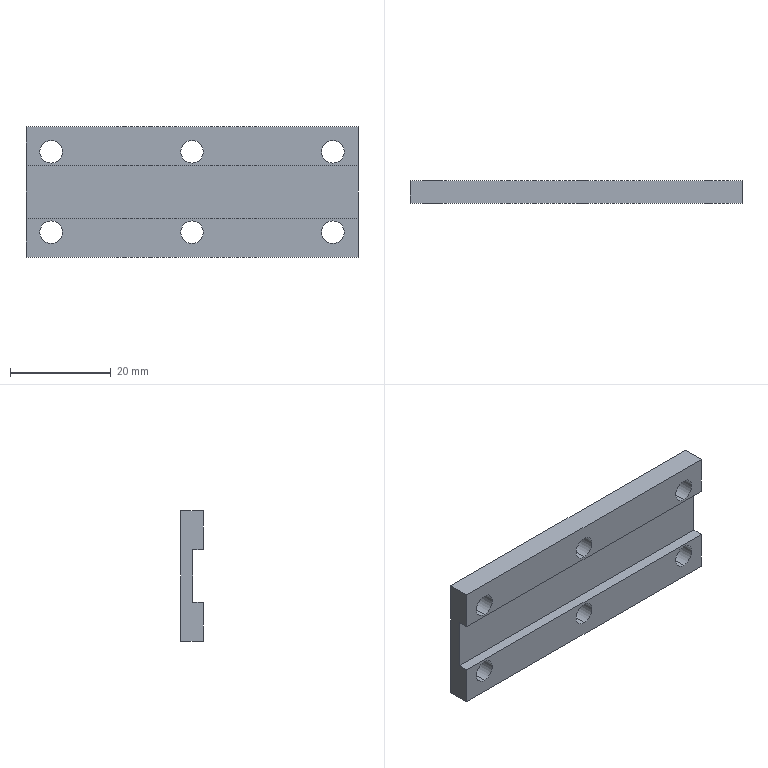Part | SolidWorks | features BaseBody 1 | 1 solid | 22 faces | box 66 x 4.5 x 26 mm | volume 5837 mm3 | cylinder 12 | plane 10 | commonest cylinder face diameters 4.5 x12
STEP:
#1=CARTESIAN_POINT('',(0.,4.7,5.75));
#2=VERTEX_POINT('',#1);
#3=CARTESIAN_POINT('',(0.,4.7,10.25));
#4=VERTEX_POINT('',#3);
#5=CARTESIAN_POINT('',(0.,4.7,8.));
#6=DIRECTION('',(0.,1.,0.));
#7=DIRECTION('',(0.,0.,1.));
#8=AXIS2_PLACEMENT_3D('',#5,#6,#7);
#9=CIRCLE('',#8,2.25);
#10=EDGE_CURVE('',#2,#4,#9,.T.);
#11=ORIENTED_EDGE('',*,*,#10,.F.);
#12=CARTESIAN_POINT('',(0.,9.2,5.75));
#13=VERTEX_POINT('',#12);
#14=CARTESIAN_POINT('',(0.,4.7,5.75));
#15=DIRECTION('',(0.,1.,0.));
#16=VECTOR('',#15,1000.);
#17=LINE('',#14,#16);
#18=EDGE_CURVE('',#2,#13,#17,.T.);
#19=ORIENTED_EDGE('',*,*,#18,.T.);
#20=CARTESIAN_POINT('',(0.,9.2,10.25));
#21=VERTEX_POINT('',#20);
#22=CARTESIAN_POINT('',(0.,9.2,8.));
#23=DIRECTION('',(0.,1.,0.));
#24=DIRECTION('',(0.,0.,1.));
#25=AXIS2_PLACEMENT_3D('',#22,#23,#24);
#26=CIRCLE('',#25,2.25);
#27=EDGE_CURVE('',#13,#21,#26,.T.);
#28=ORIENTED_EDGE('',*,*,#27,.T.);
#29=CARTESIAN_POINT('',(0.,4.7,10.25));
#30=DIRECTION('',(0.,1.,0.));
#31=VECTOR('',#30,1000.);
#32=LINE('',#29,#31);
#33=EDGE_CURVE('',#4,#21,#32,.T.);
#34=ORIENTED_EDGE('',*,*,#33,.F.);
#35=EDGE_LOOP('',(#11,#19,#28,#34));
#36=FACE_OUTER_BOUND('',#35,.T.);
#37=CARTESIAN_POINT('',(0.,4.7,8.));
#38=DIRECTION('',(0.,1.,0.));
#39=DIRECTION('',(0.,0.,1.));
#40=AXIS2_PLACEMENT_3D('',#37,#38,#39);
#41=CYLINDRICAL_SURFACE('',#40,2.25);
#42=ADVANCED_FACE('',(#36),#41,.F.);
#43=CARTESIAN_POINT('',(0.,4.7,-10.25));
#44=VERTEX_POINT('',#43);
#45=CARTESIAN_POINT('',(0.,4.7,-5.75));
#46=VERTEX_POINT('',#45);
#47=CARTESIAN_POINT('',(0.,4.7,-8.));
#48=DIRECTION('',(0.,1.,0.));
#49=DIRECTION('',(0.,0.,1.));
#50=AXIS2_PLACEMENT_3D('',#47,#48,#49);
#51=CIRCLE('',#50,2.25);
#52=EDGE_CURVE('',#44,#46,#51,.T.);
#53=ORIENTED_EDGE('',*,*,#52,.F.);
#54=CARTESIAN_POINT('',(0.,9.2,-10.25));
#55=VERTEX_POINT('',#54);
#56=CARTESIAN_POINT('',(0.,4.7,-10.25));
#57=DIRECTION('',(0.,1.,0.));
#58=VECTOR('',#57,1000.);
#59=LINE('',#56,#58);
#60=EDGE_CURVE('',#44,#55,#59,.T.);
#61=ORIENTED_EDGE('',*,*,#60,.T.);
#62=CARTESIAN_POINT('',(0.,9.2,-5.75));
#63=VERTEX_POINT('',#62);
#64=CARTESIAN_POINT('',(0.,9.2,-8.));
#65=DIRECTION('',(0.,1.,0.));
#66=DIRECTION('',(0.,0.,1.));
#67=AXIS2_PLACEMENT_3D('',#64,#65,#66);
#68=CIRCLE('',#67,2.25);
#69=EDGE_CURVE('',#55,#63,#68,.T.);
#70=ORIENTED_EDGE('',*,*,#69,.T.);
#71=CARTESIAN_POINT('',(0.,4.7,-5.75));
#72=DIRECTION('',(0.,1.,0.));
#73=VECTOR('',#72,1000.);
#74=LINE('',#71,#73);
#75=EDGE_CURVE('',#46,#63,#74,.T.);
#76=ORIENTED_EDGE('',*,*,#75,.F.);
#77=EDGE_LOOP('',(#53,#61,#70,#76));
#78=FACE_OUTER_BOUND('',#77,.T.);
#79=CARTESIAN_POINT('',(0.,4.7,-8.));
#80=DIRECTION('',(0.,1.,0.));
#81=DIRECTION('',(0.,0.,1.));
#82=AXIS2_PLACEMENT_3D('',#79,#80,#81);
#83=CYLINDRICAL_SURFACE('',#82,2.25);
#84=ADVANCED_FACE('',(#78),#83,.F.);
#85=CARTESIAN_POINT('',(28.,4.7,5.75));
#86=VERTEX_POINT('',#85);
#87=CARTESIAN_POINT('',(28.,4.7,10.25));
#88=VERTEX_POINT('',#87);
#89=CARTESIAN_POINT('',(28.,4.7,8.));
#90=DIRECTION('',(0.,1.,0.));
#91=DIRECTION('',(0.,0.,1.));
#92=AXIS2_PLACEMENT_3D('',#89,#90,#91);
#93=CIRCLE('',#92,2.25);
#94=EDGE_CURVE('',#86,#88,#93,.T.);
#95=ORIENTED_EDGE('',*,*,#94,.F.);
#96=CARTESIAN_POINT('',(28.,9.2,5.75));
#97=VERTEX_POINT('',#96);
#98=CARTESIAN_POINT('',(28.,4.7,5.75));
#99=DIRECTION('',(0.,1.,0.));
#100=VECTOR('',#99,1000.);
#101=LINE('',#98,#100);
#102=EDGE_CURVE('',#86,#97,#101,.T.);
#103=ORIENTED_EDGE('',*,*,#102,.T.);
#104=CARTESIAN_POINT('',(28.,9.2,10.25));
#105=VERTEX_POINT('',#104);
#106=CARTESIAN_POINT('',(28.,9.2,8.));
#107=DIRECTION('',(0.,1.,0.));
#108=DIRECTION('',(0.,0.,1.));
#109=AXIS2_PLACEMENT_3D('',#106,#107,#108);
#110=CIRCLE('',#109,2.25);
#111=EDGE_CURVE('',#97,#105,#110,.T.);
#112=ORIENTED_EDGE('',*,*,#111,.T.);
#113=CARTESIAN_POINT('',(28.,4.7,10.25));
#114=DIRECTION('',(0.,1.,0.));
#115=VECTOR('',#114,1000.);
#116=LINE('',#113,#115);
#117=EDGE_CURVE('',#88,#105,#116,.T.);
#118=ORIENTED_EDGE('',*,*,#117,.F.);
#119=EDGE_LOOP('',(#95,#103,#112,#118));
#120=FACE_OUTER_BOUND('',#119,.T.);
#121=CARTESIAN_POINT('',(28.,4.7,8.));
#122=DIRECTION('',(0.,1.,0.));
#123=DIRECTION('',(0.,0.,1.));
#124=AXIS2_PLACEMENT_3D('',#121,#122,#123);
#125=CYLINDRICAL_SURFACE('',#124,2.25);
#126=ADVANCED_FACE('',(#120),#125,.F.);
#127=CARTESIAN_POINT('',(28.,4.7,-10.25));
#128=VERTEX_POINT('',#127);
#129=CARTESIAN_POINT('',(28.,4.7,-5.75));
#130=VERTEX_POINT('',#129);
#131=CARTESIAN_POINT('',(28.,4.7,-8.));
#132=DIRECTION('',(0.,1.,0.));
#133=DIRECTION('',(0.,0.,1.));
#134=AXIS2_PLACEMENT_3D('',#131,#132,#133);
#135=CIRCLE('',#134,2.25);
#136=EDGE_CURVE('',#128,#130,#135,.T.);
#137=ORIENTED_EDGE('',*,*,#136,.F.);
#138=CARTESIAN_POINT('',(28.,9.2,-10.25));
#139=VERTEX_POINT('',#138);
#140=CARTESIAN_POINT('',(28.,4.7,-10.25));
#141=DIRECTION('',(0.,1.,0.));
#142=VECTOR('',#141,1000.);
#143=LINE('',#140,#142);
#144=EDGE_CURVE('',#128,#139,#143,.T.);
#145=ORIENTED_EDGE('',*,*,#144,.T.);
#146=CARTESIAN_POINT('',(28.,9.2,-5.75));
#147=VERTEX_POINT('',#146);
#148=CARTESIAN_POINT('',(28.,9.2,-8.));
#149=DIRECTION('',(0.,1.,0.));
#150=DIRECTION('',(0.,0.,1.));
#151=AXIS2_PLACEMENT_3D('',#148,#149,#150);
#152=CIRCLE('',#151,2.25);
#153=EDGE_CURVE('',#139,#147,#152,.T.);
#154=ORIENTED_EDGE('',*,*,#153,.T.);
#155=CARTESIAN_POINT('',(28.,4.7,-5.75));
#156=DIRECTION('',(0.,1.,0.));
#157=VECTOR('',#156,1000.);
#158=LINE('',#155,#157);
#159=EDGE_CURVE('',#130,#147,#158,.T.);
#160=ORIENTED_EDGE('',*,*,#159,.F.);
#161=EDGE_LOOP('',(#137,#145,#154,#160));
#162=FACE_OUTER_BOUND('',#161,.T.);
#163=CARTESIAN_POINT('',(28.,4.7,-8.));
#164=DIRECTION('',(0.,1.,0.));
#165=DIRECTION('',(0.,0.,1.));
#166=AXIS2_PLACEMENT_3D('',#163,#164,#165);
#167=CYLINDRICAL_SURFACE('',#166,2.25);
#168=ADVANCED_FACE('',(#162),#167,.F.);
#169=CARTESIAN_POINT('',(56.,4.7,5.75));
#170=VERTEX_POINT('',#169);
#171=CARTESIAN_POINT('',(56.,4.7,10.25));
#172=VERTEX_POINT('',#171);
#173=CARTESIAN_POINT('',(56.,4.7,8.));
#174=DIRECTION('',(0.,1.,0.));
#175=DIRECTION('',(0.,0.,1.));
#176=AXIS2_PLACEMENT_3D('',#173,#174,#175);
#177=CIRCLE('',#176,2.25);
#178=EDGE_CURVE('',#170,#172,#177,.T.);
#179=ORIENTED_EDGE('',*,*,#178,.F.);
#180=CARTESIAN_POINT('',(56.,9.2,5.75));
#181=VERTEX_POINT('',#180);
#182=CARTESIAN_POINT('',(56.,4.7,5.75));
#183=DIRECTION('',(0.,1.,0.));
#184=VECTOR('',#183,1000.);
#185=LINE('',#182,#184);
#186=EDGE_CURVE('',#170,#181,#185,.T.);
#187=ORIENTED_EDGE('',*,*,#186,.T.);
#188=CARTESIAN_POINT('',(56.,9.2,10.25));
#189=VERTEX_POINT('',#188);
#190=CARTESIAN_POINT('',(56.,9.2,8.));
#191=DIRECTION('',(0.,1.,0.));
#192=DIRECTION('',(0.,0.,1.));
#193=AXIS2_PLACEMENT_3D('',#190,#191,#192);
#194=CIRCLE('',#193,2.25);
#195=EDGE_CURVE('',#181,#189,#194,.T.);
#196=ORIENTED_EDGE('',*,*,#195,.T.);
#197=CARTESIAN_POINT('',(56.,4.7,10.25));
#198=DIRECTION('',(0.,1.,0.));
#199=VECTOR('',#198,1000.);
#200=LINE('',#197,#199);
#201=EDGE_CURVE('',#172,#189,#200,.T.);
#202=ORIENTED_EDGE('',*,*,#201,.F.);
#203=EDGE_LOOP('',(#179,#187,#196,#202));
#204=FACE_OUTER_BOUND('',#203,.T.);
#205=CARTESIAN_POINT('',(56.,4.7,8.));
#206=DIRECTION('',(0.,1.,0.));
#207=DIRECTION('',(0.,0.,1.));
#208=AXIS2_PLACEMENT_3D('',#205,#206,#207);
#209=CYLINDRICAL_SURFACE('',#208,2.25);
#210=ADVANCED_FACE('',(#204),#209,.F.);
#211=CARTESIAN_POINT('',(56.,4.7,-10.25));
#212=VERTEX_POINT('',#211);
#213=CARTESIAN_POINT('',(56.,4.7,-5.75));
#214=VERTEX_POINT('',#213);
#215=CARTESIAN_POINT('',(56.,4.7,-8.));
#216=DIRECTION('',(0.,1.,0.));
#217=DIRECTION('',(0.,0.,1.));
#218=AXIS2_PLACEMENT_3D('',#215,#216,#217);
#219=CIRCLE('',#218,2.25);
#220=EDGE_CURVE('',#212,#214,#219,.T.);
#221=ORIENTED_EDGE('',*,*,#220,.F.);
#222=CARTESIAN_POINT('',(56.,9.2,-10.25));
#223=VERTEX_POINT('',#222);
#224=CARTESIAN_POINT('',(56.,4.7,-10.25));
#225=DIRECTION('',(0.,1.,0.));
#226=VECTOR('',#225,1000.);
#227=LINE('',#224,#226);
#228=EDGE_CURVE('',#212,#223,#227,.T.);
#229=ORIENTED_EDGE('',*,*,#228,.T.);
#230=CARTESIAN_POINT('',(56.,9.2,-5.75));
#231=VERTEX_POINT('',#230);
#232=CARTESIAN_POINT('',(56.,9.2,-8.));
#233=DIRECTION('',(0.,1.,0.));
#234=DIRECTION('',(0.,0.,1.));
#235=AXIS2_PLACEMENT_3D('',#232,#233,#234);
#236=CIRCLE('',#235,2.25);
#237=EDGE_CURVE('',#223,#231,#236,.T.);
#238=ORIENTED_EDGE('',*,*,#237,.T.);
#239=CARTESIAN_POINT('',(56.,4.7,-5.75));
#240=DIRECTION('',(0.,1.,0.));
#241=VECTOR('',#240,1000.);
#242=LINE('',#239,#241);
#243=EDGE_CURVE('',#214,#231,#242,.T.);
#244=ORIENTED_EDGE('',*,*,#243,.F.);
#245=EDGE_LOOP('',(#221,#229,#238,#244));
#246=FACE_OUTER_BOUND('',#245,.T.);
#247=CARTESIAN_POINT('',(56.,4.7,-8.));
#248=DIRECTION('',(0.,1.,0.));
#249=DIRECTION('',(0.,0.,1.));
#250=AXIS2_PLACEMENT_3D('',#247,#248,#249);
#251=CYLINDRICAL_SURFACE('',#250,2.25);
#252=ADVANCED_FACE('',(#246),#251,.F.);
#253=CARTESIAN_POINT('',(61.,9.2,13.));
#254=VERTEX_POINT('',#253);
#255=CARTESIAN_POINT('',(-5.,9.2,13.));
#256=VERTEX_POINT('',#255);
#257=CARTESIAN_POINT('',(61.,9.2,13.));
#258=DIRECTION('',(-1.,0.,0.));
#259=VECTOR('',#258,1000.);
#260=LINE('',#257,#259);
#261=EDGE_CURVE('',#254,#256,#260,.T.);
#262=ORIENTED_EDGE('',*,*,#261,.F.);
#263=CARTESIAN_POINT('',(61.,9.2,-13.));
#264=VERTEX_POINT('',#263);
#265=CARTESIAN_POINT('',(61.,9.2,13.));
#266=DIRECTION('',(0.,0.,1.));
#267=VECTOR('',#266,1000.);
#268=LINE('',#265,#267);
#269=EDGE_CURVE('',#264,#254,#268,.T.);
#270=ORIENTED_EDGE('',*,*,#269,.F.);
#271=CARTESIAN_POINT('',(-5.,9.2,-13.));
#272=VERTEX_POINT('',#271);
#273=CARTESIAN_POINT('',(61.,9.2,-13.));
#274=DIRECTION('',(1.,0.,0.));
#275=VECTOR('',#274,1000.);
#276=LINE('',#273,#275);
#277=EDGE_CURVE('',#272,#264,#276,.T.);
#278=ORIENTED_EDGE('',*,*,#277,.F.);
#279=CARTESIAN_POINT('',(-5.,9.2,13.));
#280=DIRECTION('',(0.,0.,-1.));
#281=VECTOR('',#280,1000.);
#282=LINE('',#279,#281);
#283=EDGE_CURVE('',#256,#272,#282,.T.);
#284=ORIENTED_EDGE('',*,*,#283,.F.);
#285=EDGE_LOOP('',(#262,#270,#278,#284));
#286=FACE_OUTER_BOUND('',#285,.T.);
#287=CARTESIAN_POINT('',(0.,9.2,8.));
#288=DIRECTION('',(0.,1.,0.));
#289=DIRECTION('',(0.,0.,1.));
#290=AXIS2_PLACEMENT_3D('',#287,#288,#289);
#291=CIRCLE('',#290,2.25);
#292=EDGE_CURVE('',#21,#13,#291,.T.);
#293=ORIENTED_EDGE('',*,*,#292,.F.);
#294=ORIENTED_EDGE('',*,*,#27,.F.);
#295=EDGE_LOOP('',(#293,#294));
#296=FACE_BOUND('',#295,.T.);
#297=CARTESIAN_POINT('',(0.,9.2,-8.));
#298=DIRECTION('',(0.,1.,0.));
#299=DIRECTION('',(0.,0.,1.));
#300=AXIS2_PLACEMENT_3D('',#297,#298,#299);
#301=CIRCLE('',#300,2.25);
#302=EDGE_CURVE('',#63,#55,#301,.T.);
#303=ORIENTED_EDGE('',*,*,#302,.F.);
#304=ORIENTED_EDGE('',*,*,#69,.F.);
#305=EDGE_LOOP('',(#303,#304));
#306=FACE_BOUND('',#305,.T.);
#307=CARTESIAN_POINT('',(28.,9.2,8.));
#308=DIRECTION('',(0.,1.,0.));
#309=DIRECTION('',(0.,0.,1.));
#310=AXIS2_PLACEMENT_3D('',#307,#308,#309);
#311=CIRCLE('',#310,2.25);
#312=EDGE_CURVE('',#105,#97,#311,.T.);
#313=ORIENTED_EDGE('',*,*,#312,.F.);
#314=ORIENTED_EDGE('',*,*,#111,.F.);
#315=EDGE_LOOP('',(#313,#314));
#316=FACE_BOUND('',#315,.T.);
#317=CARTESIAN_POINT('',(28.,9.2,-8.));
#318=DIRECTION('',(0.,1.,0.));
#319=DIRECTION('',(0.,0.,1.));
#320=AXIS2_PLACEMENT_3D('',#317,#318,#319);
#321=CIRCLE('',#320,2.25);
#322=EDGE_CURVE('',#147,#139,#321,.T.);
#323=ORIENTED_EDGE('',*,*,#322,.F.);
#324=ORIENTED_EDGE('',*,*,#153,.F.);
#325=EDGE_LOOP('',(#323,#324));
#326=FACE_BOUND('',#325,.T.);
#327=CARTESIAN_POINT('',(56.,9.2,8.));
#328=DIRECTION('',(0.,1.,0.));
#329=DIRECTION('',(0.,0.,1.));
#330=AXIS2_PLACEMENT_3D('',#327,#328,#329);
#331=CIRCLE('',#330,2.25);
#332=EDGE_CURVE('',#189,#181,#331,.T.);
#333=ORIENTED_EDGE('',*,*,#332,.F.);
#334=ORIENTED_EDGE('',*,*,#195,.F.);
#335=EDGE_LOOP('',(#333,#334));
#336=FACE_BOUND('',#335,.T.);
#337=CARTESIAN_POINT('',(56.,9.2,-8.));
#338=DIRECTION('',(0.,1.,0.));
#339=DIRECTION('',(0.,0.,1.));
#340=AXIS2_PLACEMENT_3D('',#337,#338,#339);
#341=CIRCLE('',#340,2.25);
#342=EDGE_CURVE('',#231,#223,#341,.T.);
#343=ORIENTED_EDGE('',*,*,#342,.F.);
#344=ORIENTED_EDGE('',*,*,#237,.F.);
#345=EDGE_LOOP('',(#343,#344));
#346=FACE_BOUND('',#345,.T.);
#347=CARTESIAN_POINT('',(61.,9.2,13.));
#348=DIRECTION('',(0.,-1.,0.));
#349=DIRECTION('',(0.,0.,-1.));
#350=AXIS2_PLACEMENT_3D('',#347,#348,#349);
#351=PLANE('',#350);
#352=ADVANCED_FACE('',(#286,#296,#306,#316,#326,#336,#346),#351,.F.);
#353=ORIENTED_EDGE('',*,*,#283,.T.);
#354=CARTESIAN_POINT('',(-5.,4.7,-13.));
#355=VERTEX_POINT('',#354);
#356=CARTESIAN_POINT('',(-5.,0.,-13.));
#357=DIRECTION('',(0.,1.,0.));
#358=VECTOR('',#357,1000.);
#359=LINE('',#356,#358);
#360=EDGE_CURVE('',#355,#272,#359,.T.);
#361=ORIENTED_EDGE('',*,*,#360,.F.);
#362=CARTESIAN_POINT('',(-5.,4.7,-5.25));
#363=VERTEX_POINT('',#362);
#364=CARTESIAN_POINT('',(-5.,4.7,0.));
#365=DIRECTION('',(0.,0.,-1.));
#366=VECTOR('',#365,1000.);
#367=LINE('',#364,#366);
#368=EDGE_CURVE('',#363,#355,#367,.T.);
#369=ORIENTED_EDGE('',*,*,#368,.F.);
#370=CARTESIAN_POINT('',(-5.,6.8,-5.25));
#371=VERTEX_POINT('',#370);
#372=CARTESIAN_POINT('',(-5.,0.,-5.25));
#373=DIRECTION('',(0.,-1.,0.));
#374=VECTOR('',#373,1000.);
#375=LINE('',#372,#374);
#376=EDGE_CURVE('',#371,#363,#375,.T.);
#377=ORIENTED_EDGE('',*,*,#376,.F.);
#378=CARTESIAN_POINT('',(-5.,6.8,5.25));
#379=VERTEX_POINT('',#378);
#380=CARTESIAN_POINT('',(-5.,6.8,0.));
#381=DIRECTION('',(0.,0.,-1.));
#382=VECTOR('',#381,1000.);
#383=LINE('',#380,#382);
#384=EDGE_CURVE('',#379,#371,#383,.T.);
#385=ORIENTED_EDGE('',*,*,#384,.F.);
#386=CARTESIAN_POINT('',(-5.,4.7,5.25));
#387=VERTEX_POINT('',#386);
#388=CARTESIAN_POINT('',(-5.,0.,5.25));
#389=DIRECTION('',(0.,1.,0.));
#390=VECTOR('',#389,1000.);
#391=LINE('',#388,#390);
#392=EDGE_CURVE('',#387,#379,#391,.T.);
#393=ORIENTED_EDGE('',*,*,#392,.F.);
#394=CARTESIAN_POINT('',(-5.,4.7,13.));
#395=VERTEX_POINT('',#394);
#396=CARTESIAN_POINT('',(-5.,4.7,0.));
#397=DIRECTION('',(0.,0.,-1.));
#398=VECTOR('',#397,1000.);
#399=LINE('',#396,#398);
#400=EDGE_CURVE('',#395,#387,#399,.T.);
#401=ORIENTED_EDGE('',*,*,#400,.F.);
#402=CARTESIAN_POINT('',(-5.,0.,13.));
#403=DIRECTION('',(0.,-1.,0.));
#404=VECTOR('',#403,1000.);
#405=LINE('',#402,#404);
#406=EDGE_CURVE('',#256,#395,#405,.T.);
#407=ORIENTED_EDGE('',*,*,#406,.F.);
#408=EDGE_LOOP('',(#353,#361,#369,#377,#385,#393,#401,#407));
#409=FACE_OUTER_BOUND('',#408,.T.);
#410=CARTESIAN_POINT('',(-5.,0.,0.));
#411=DIRECTION('',(1.,0.,0.));
#412=DIRECTION('',(0.,0.,-1.));
#413=AXIS2_PLACEMENT_3D('',#410,#411,#412);
#414=PLANE('',#413);
#415=ADVANCED_FACE('',(#409),#414,.F.);
#416=CARTESIAN_POINT('',(61.,4.7,13.));
#417=VERTEX_POINT('',#416);
#418=CARTESIAN_POINT('',(61.,4.7,13.));
#419=DIRECTION('',(-1.,0.,0.));
#420=VECTOR('',#419,1000.);
#421=LINE('',#418,#420);
#422=EDGE_CURVE('',#417,#395,#421,.T.);
#423=ORIENTED_EDGE('',*,*,#422,.F.);
#424=CARTESIAN_POINT('',(61.,9.2,13.));
#425=DIRECTION('',(0.,-1.,0.));
#426=VECTOR('',#425,1000.);
#427=LINE('',#424,#426);
#428=EDGE_CURVE('',#254,#417,#427,.T.);
#429=ORIENTED_EDGE('',*,*,#428,.F.);
#430=ORIENTED_EDGE('',*,*,#261,.T.);
#431=ORIENTED_EDGE('',*,*,#406,.T.);
#432=EDGE_LOOP('',(#423,#429,#430,#431));
#433=FACE_OUTER_BOUND('',#432,.T.);
#434=CARTESIAN_POINT('',(61.,9.2,13.));
#435=DIRECTION('',(0.,0.,-1.));
#436=DIRECTION('',(-1.,0.,0.));
#437=AXIS2_PLACEMENT_3D('',#434,#435,#436);
#438=PLANE('',#437);
#439=ADVANCED_FACE('',(#433),#438,.F.);
#440=CARTESIAN_POINT('',(61.,4.7,-13.));
#441=VERTEX_POINT('',#440);
#442=CARTESIAN_POINT('',(61.,0.,-13.));
#443=DIRECTION('',(0.,1.,0.));
#444=VECTOR('',#443,1000.);
#445=LINE('',#442,#444);
#446=EDGE_CURVE('',#441,#264,#445,.T.);
#447=ORIENTED_EDGE('',*,*,#446,.T.);
#448=ORIENTED_EDGE('',*,*,#269,.T.);
#449=ORIENTED_EDGE('',*,*,#428,.T.);
#450=CARTESIAN_POINT('',(61.,4.7,5.25));
#451=VERTEX_POINT('',#450);
#452=CARTESIAN_POINT('',(61.,4.7,0.));
#453=DIRECTION('',(0.,0.,-1.));
#454=VECTOR('',#453,1000.);
#455=LINE('',#452,#454);
#456=EDGE_CURVE('',#417,#451,#455,.T.);
#457=ORIENTED_EDGE('',*,*,#456,.T.);
#458=CARTESIAN_POINT('',(61.,6.8,5.25));
#459=VERTEX_POINT('',#458);
#460=CARTESIAN_POINT('',(61.,0.,5.25));
#461=DIRECTION('',(0.,1.,0.));
#462=VECTOR('',#461,1000.);
#463=LINE('',#460,#462);
#464=EDGE_CURVE('',#451,#459,#463,.T.);
#465=ORIENTED_EDGE('',*,*,#464,.T.);
#466=CARTESIAN_POINT('',(61.,6.8,-5.25));
#467=VERTEX_POINT('',#466);
#468=CARTESIAN_POINT('',(61.,6.8,0.));
#469=DIRECTION('',(0.,0.,-1.));
#470=VECTOR('',#469,1000.);
#471=LINE('',#468,#470);
#472=EDGE_CURVE('',#459,#467,#471,.T.);
#473=ORIENTED_EDGE('',*,*,#472,.T.);
#474=CARTESIAN_POINT('',(61.,4.7,-5.25));
#475=VERTEX_POINT('',#474);
#476=CARTESIAN_POINT('',(61.,0.,-5.25));
#477=DIRECTION('',(0.,-1.,0.));
#478=VECTOR('',#477,1000.);
#479=LINE('',#476,#478);
#480=EDGE_CURVE('',#467,#475,#479,.T.);
#481=ORIENTED_EDGE('',*,*,#480,.T.);
#482=CARTESIAN_POINT('',(61.,4.7,0.));
#483=DIRECTION('',(0.,0.,-1.));
#484=VECTOR('',#483,1000.);
#485=LINE('',#482,#484);
#486=EDGE_CURVE('',#475,#441,#485,.T.);
#487=ORIENTED_EDGE('',*,*,#486,.T.);
#488=EDGE_LOOP('',(#447,#448,#449,#457,#465,#473,#481,#487));
#489=FACE_OUTER_BOUND('',#488,.T.);
#490=CARTESIAN_POINT('',(61.,0.,0.));
#491=DIRECTION('',(1.,0.,0.));
#492=DIRECTION('',(0.,0.,-1.));
#493=AXIS2_PLACEMENT_3D('',#490,#491,#492);
#494=PLANE('',#493);
#495=ADVANCED_FACE('',(#489),#494,.T.);
#496=ORIENTED_EDGE('',*,*,#277,.T.);
#497=ORIENTED_EDGE('',*,*,#446,.F.);
#498=CARTESIAN_POINT('',(61.,4.7,-13.));
#499=DIRECTION('',(1.,0.,0.));
#500=VECTOR('',#499,1000.);
#501=LINE('',#498,#500);
#502=EDGE_CURVE('',#355,#441,#501,.T.);
#503=ORIENTED_EDGE('',*,*,#502,.F.);
#504=ORIENTED_EDGE('',*,*,#360,.T.);
#505=EDGE_LOOP('',(#496,#497,#503,#504));
#506=FACE_OUTER_BOUND('',#505,.T.);
#507=CARTESIAN_POINT('',(61.,9.2,-13.));
#508=DIRECTION('',(0.,0.,1.));
#509=DIRECTION('',(1.,0.,0.));
#510=AXIS2_PLACEMENT_3D('',#507,#508,#509);
#511=PLANE('',#510);
#512=ADVANCED_FACE('',(#506),#511,.F.);
#513=ORIENTED_EDGE('',*,*,#18,.F.);
#514=CARTESIAN_POINT('',(0.,4.7,8.));
#515=DIRECTION('',(0.,1.,0.));
#516=DIRECTION('',(0.,0.,1.));
#517=AXIS2_PLACEMENT_3D('',#514,#515,#516);
#518=CIRCLE('',#517,2.25);
#519=EDGE_CURVE('',#4,#2,#518,.T.);
#520=ORIENTED_EDGE('',*,*,#519,.F.);
#521=ORIENTED_EDGE('',*,*,#33,.T.);
#522=ORIENTED_EDGE('',*,*,#292,.T.);
#523=EDGE_LOOP('',(#513,#520,#521,#522));
#524=FACE_OUTER_BOUND('',#523,.T.);
#525=CARTESIAN_POINT('',(0.,4.7,8.));
#526=DIRECTION('',(0.,1.,0.));
#527=DIRECTION('',(0.,0.,1.));
#528=AXIS2_PLACEMENT_3D('',#525,#526,#527);
#529=CYLINDRICAL_SURFACE('',#528,2.25);
#530=ADVANCED_FACE('',(#524),#529,.F.);
#531=ORIENTED_EDGE('',*,*,#60,.F.);
#532=CARTESIAN_POINT('',(0.,4.7,-8.));
#533=DIRECTION('',(0.,1.,0.));
#534=DIRECTION('',(0.,0.,1.));
#535=AXIS2_PLACEMENT_3D('',#532,#533,#534);
#536=CIRCLE('',#535,2.25);
#537=EDGE_CURVE('',#46,#44,#536,.T.);
#538=ORIENTED_EDGE('',*,*,#537,.F.);
#539=ORIENTED_EDGE('',*,*,#75,.T.);
#540=ORIENTED_EDGE('',*,*,#302,.T.);
#541=EDGE_LOOP('',(#531,#538,#539,#540));
#542=FACE_OUTER_BOUND('',#541,.T.);
#543=CARTESIAN_POINT('',(0.,4.7,-8.));
#544=DIRECTION('',(0.,1.,0.));
#545=DIRECTION('',(0.,0.,1.));
#546=AXIS2_PLACEMENT_3D('',#543,#544,#545);
#547=CYLINDRICAL_SURFACE('',#546,2.25);
#548=ADVANCED_FACE('',(#542),#547,.F.);
#549=ORIENTED_EDGE('',*,*,#102,.F.);
#550=CARTESIAN_POINT('',(28.,4.7,8.));
#551=DIRECTION('',(0.,1.,0.));
#552=DIRECTION('',(0.,0.,1.));
#553=AXIS2_PLACEMENT_3D('',#550,#551,#552);
#554=CIRCLE('',#553,2.25);
#555=EDGE_CURVE('',#88,#86,#554,.T.);
#556=ORIENTED_EDGE('',*,*,#555,.F.);
#557=ORIENTED_EDGE('',*,*,#117,.T.);
#558=ORIENTED_EDGE('',*,*,#312,.T.);
#559=EDGE_LOOP('',(#549,#556,#557,#558));
#560=FACE_OUTER_BOUND('',#559,.T.);
#561=CARTESIAN_POINT('',(28.,4.7,8.));
#562=DIRECTION('',(0.,1.,0.));
#563=DIRECTION('',(0.,0.,1.));
#564=AXIS2_PLACEMENT_3D('',#561,#562,#563);
#565=CYLINDRICAL_SURFACE('',#564,2.25);
#566=ADVANCED_FACE('',(#560),#565,.F.);
#567=ORIENTED_EDGE('',*,*,#144,.F.);
#568=CARTESIAN_POINT('',(28.,4.7,-8.));
#569=DIRECTION('',(0.,1.,0.));
#570=DIRECTION('',(0.,0.,1.));
#571=AXIS2_PLACEMENT_3D('',#568,#569,#570);
#572=CIRCLE('',#571,2.25);
#573=EDGE_CURVE('',#130,#128,#572,.T.);
#574=ORIENTED_EDGE('',*,*,#573,.F.);
#575=ORIENTED_EDGE('',*,*,#159,.T.);
#576=ORIENTED_EDGE('',*,*,#322,.T.);
#577=EDGE_LOOP('',(#567,#574,#575,#576));
#578=FACE_OUTER_BOUND('',#577,.T.);
#579=CARTESIAN_POINT('',(28.,4.7,-8.));
#580=DIRECTION('',(0.,1.,0.));
#581=DIRECTION('',(0.,0.,1.));
#582=AXIS2_PLACEMENT_3D('',#579,#580,#581);
#583=CYLINDRICAL_SURFACE('',#582,2.25);
#584=ADVANCED_FACE('',(#578),#583,.F.);
#585=ORIENTED_EDGE('',*,*,#186,.F.);
#586=CARTESIAN_POINT('',(56.,4.7,8.));
#587=DIRECTION('',(0.,1.,0.));
#588=DIRECTION('',(0.,0.,1.));
#589=AXIS2_PLACEMENT_3D('',#586,#587,#588);
#590=CIRCLE('',#589,2.25);
#591=EDGE_CURVE('',#172,#170,#590,.T.);
#592=ORIENTED_EDGE('',*,*,#591,.F.);
#593=ORIENTED_EDGE('',*,*,#201,.T.);
#594=ORIENTED_EDGE('',*,*,#332,.T.);
#595=EDGE_LOOP('',(#585,#592,#593,#594));
#596=FACE_OUTER_BOUND('',#595,.T.);
#597=CARTESIAN_POINT('',(56.,4.7,8.));
#598=DIRECTION('',(0.,1.,0.));
#599=DIRECTION('',(0.,0.,1.));
#600=AXIS2_PLACEMENT_3D('',#597,#598,#599);
#601=CYLINDRICAL_SURFACE('',#600,2.25);
#602=ADVANCED_FACE('',(#596),#601,.F.);
#603=ORIENTED_EDGE('',*,*,#228,.F.);
#604=CARTESIAN_POINT('',(56.,4.7,-8.));
#605=DIRECTION('',(0.,1.,0.));
#606=DIRECTION('',(0.,0.,1.));
#607=AXIS2_PLACEMENT_3D('',#604,#605,#606);
#608=CIRCLE('',#607,2.25);
#609=EDGE_CURVE('',#214,#212,#608,.T.);
#610=ORIENTED_EDGE('',*,*,#609,.F.);
#611=ORIENTED_EDGE('',*,*,#243,.T.);
#612=ORIENTED_EDGE('',*,*,#342,.T.);
#613=EDGE_LOOP('',(#603,#610,#611,#612));
#614=FACE_OUTER_BOUND('',#613,.T.);
#615=CARTESIAN_POINT('',(56.,4.7,-8.));
#616=DIRECTION('',(0.,1.,0.));
#617=DIRECTION('',(0.,0.,1.));
#618=AXIS2_PLACEMENT_3D('',#615,#616,#617);
#619=CYLINDRICAL_SURFACE('',#618,2.25);
#620=ADVANCED_FACE('',(#614),#619,.F.);
#621=ORIENTED_EDGE('',*,*,#502,.T.);
#622=ORIENTED_EDGE('',*,*,#486,.F.);
#623=CARTESIAN_POINT('',(61.,4.7,-5.25));
#624=DIRECTION('',(1.,0.,0.));
#625=VECTOR('',#624,1000.);
#626=LINE('',#623,#625);
#627=EDGE_CURVE('',#363,#475,#626,.T.);
#628=ORIENTED_EDGE('',*,*,#627,.F.);
#629=ORIENTED_EDGE('',*,*,#368,.T.);
#630=EDGE_LOOP('',(#621,#622,#628,#629));
#631=FACE_OUTER_BOUND('',#630,.T.);
#632=ORIENTED_EDGE('',*,*,#537,.T.);
#633=ORIENTED_EDGE('',*,*,#52,.T.);
#634=EDGE_LOOP('',(#632,#633));
#635=FACE_BOUND('',#634,.T.);
#636=ORIENTED_EDGE('',*,*,#573,.T.);
#637=ORIENTED_EDGE('',*,*,#136,.T.);
#638=EDGE_LOOP('',(#636,#637));
#639=FACE_BOUND('',#638,.T.);
#640=ORIENTED_EDGE('',*,*,#609,.T.);
#641=ORIENTED_EDGE('',*,*,#220,.T.);
#642=EDGE_LOOP('',(#640,#641));
#643=FACE_BOUND('',#642,.T.);
#644=CARTESIAN_POINT('',(61.,4.7,-5.25));
#645=DIRECTION('',(0.,1.,0.));
#646=DIRECTION('',(0.,0.,1.));
#647=AXIS2_PLACEMENT_3D('',#644,#645,#646);
#648=PLANE('',#647);
#649=ADVANCED_FACE('',(#631,#635,#639,#643),#648,.F.);
#650=ORIENTED_EDGE('',*,*,#627,.T.);
#651=ORIENTED_EDGE('',*,*,#480,.F.);
#652=CARTESIAN_POINT('',(61.,6.8,-5.25));
#653=DIRECTION('',(1.,0.,0.));
#654=VECTOR('',#653,1000.);
#655=LINE('',#652,#654);
#656=EDGE_CURVE('',#371,#467,#655,.T.);
#657=ORIENTED_EDGE('',*,*,#656,.F.);
#658=ORIENTED_EDGE('',*,*,#376,.T.);
#659=EDGE_LOOP('',(#650,#651,#657,#658));
#660=FACE_OUTER_BOUND('',#659,.T.);
#661=CARTESIAN_POINT('',(61.,6.8,-5.25));
#662=DIRECTION('',(0.,0.,-1.));
#663=DIRECTION('',(-1.,0.,0.));
#664=AXIS2_PLACEMENT_3D('',#661,#662,#663);
#665=PLANE('',#664);
#666=ADVANCED_FACE('',(#660),#665,.F.);
#667=ORIENTED_EDGE('',*,*,#656,.T.);
#668=ORIENTED_EDGE('',*,*,#472,.F.);
#669=CARTESIAN_POINT('',(61.,6.8,5.25));
#670=DIRECTION('',(1.,0.,0.));
#671=VECTOR('',#670,1000.);
#672=LINE('',#669,#671);
#673=EDGE_CURVE('',#379,#459,#672,.T.);
#674=ORIENTED_EDGE('',*,*,#673,.F.);
#675=ORIENTED_EDGE('',*,*,#384,.T.);
#676=EDGE_LOOP('',(#667,#668,#674,#675));
#677=FACE_OUTER_BOUND('',#676,.T.);
#678=CARTESIAN_POINT('',(61.,6.8,5.25));
#679=DIRECTION('',(0.,1.,0.));
#680=DIRECTION('',(0.,0.,1.));
#681=AXIS2_PLACEMENT_3D('',#678,#679,#680);
#682=PLANE('',#681);
#683=ADVANCED_FACE('',(#677),#682,.F.);
#684=ORIENTED_EDGE('',*,*,#673,.T.);
#685=ORIENTED_EDGE('',*,*,#464,.F.);
#686=CARTESIAN_POINT('',(61.,4.7,5.25));
#687=DIRECTION('',(1.,0.,0.));
#688=VECTOR('',#687,1000.);
#689=LINE('',#686,#688);
#690=EDGE_CURVE('',#387,#451,#689,.T.);
#691=ORIENTED_EDGE('',*,*,#690,.F.);
#692=ORIENTED_EDGE('',*,*,#392,.T.);
#693=EDGE_LOOP('',(#684,#685,#691,#692));
#694=FACE_OUTER_BOUND('',#693,.T.);
#695=CARTESIAN_POINT('',(61.,4.7,5.25));
#696=DIRECTION('',(0.,0.,1.));
#697=DIRECTION('',(1.,0.,0.));
#698=AXIS2_PLACEMENT_3D('',#695,#696,#697);
#699=PLANE('',#698);
#700=ADVANCED_FACE('',(#694),#699,.F.);
#701=ORIENTED_EDGE('',*,*,#690,.T.);
#702=ORIENTED_EDGE('',*,*,#456,.F.);
#703=ORIENTED_EDGE('',*,*,#422,.T.);
#704=ORIENTED_EDGE('',*,*,#400,.T.);
#705=EDGE_LOOP('',(#701,#702,#703,#704));
#706=FACE_OUTER_BOUND('',#705,.T.);
#707=ORIENTED_EDGE('',*,*,#519,.T.);
#708=ORIENTED_EDGE('',*,*,#10,.T.);
#709=EDGE_LOOP('',(#707,#708));
#710=FACE_BOUND('',#709,.T.);
#711=ORIENTED_EDGE('',*,*,#555,.T.);
#712=ORIENTED_EDGE('',*,*,#94,.T.);
#713=EDGE_LOOP('',(#711,#712));
#714=FACE_BOUND('',#713,.T.);
#715=ORIENTED_EDGE('',*,*,#591,.T.);
#716=ORIENTED_EDGE('',*,*,#178,.T.);
#717=EDGE_LOOP('',(#715,#716));
#718=FACE_BOUND('',#717,.T.);
#719=CARTESIAN_POINT('',(61.,4.7,13.));
#720=DIRECTION('',(0.,1.,0.));
#721=DIRECTION('',(0.,0.,1.));
#722=AXIS2_PLACEMENT_3D('',#719,#720,#721);
#723=PLANE('',#722);
#724=ADVANCED_FACE('',(#706,#710,#714,#718),#723,.F.);
#725=CLOSED_SHELL('',(#42,#84,#126,#168,#210,#252,#352,#415,#439,#495,#512,#530,#548,#566,#584,#602,#620,#649,#666,#683,#700,#724));
#726=MANIFOLD_SOLID_BREP('',#725);
#727=CARTESIAN_POINT('',(0.,0.,0.));
#728=DIRECTION('',(0.,0.,1.));
#729=DIRECTION('',(1.,0.,0.));
#730=AXIS2_PLACEMENT_3D('',#727,#728,#729);
#731=(LENGTH_UNIT()NAMED_UNIT(*)SI_UNIT(.MILLI.,.METRE.));
#732=UNCERTAINTY_MEASURE_WITH_UNIT(LENGTH_MEASURE(0.00001),#731,'','');
#733=(NAMED_UNIT(*)PLANE_ANGLE_UNIT()SI_UNIT($,.RADIAN.));
#734=(NAMED_UNIT(*)SI_UNIT($,.STERADIAN.)SOLID_ANGLE_UNIT());
#735=(GEOMETRIC_REPRESENTATION_CONTEXT(3)GLOBAL_UNCERTAINTY_ASSIGNED_CONTEXT((#732))GLOBAL_UNIT_ASSIGNED_CONTEXT((#731,#733,#734))REPRESENTATION_CONTEXT('',''));
#736=ADVANCED_BREP_SHAPE_REPRESENTATION('',(#726,#730),#735);